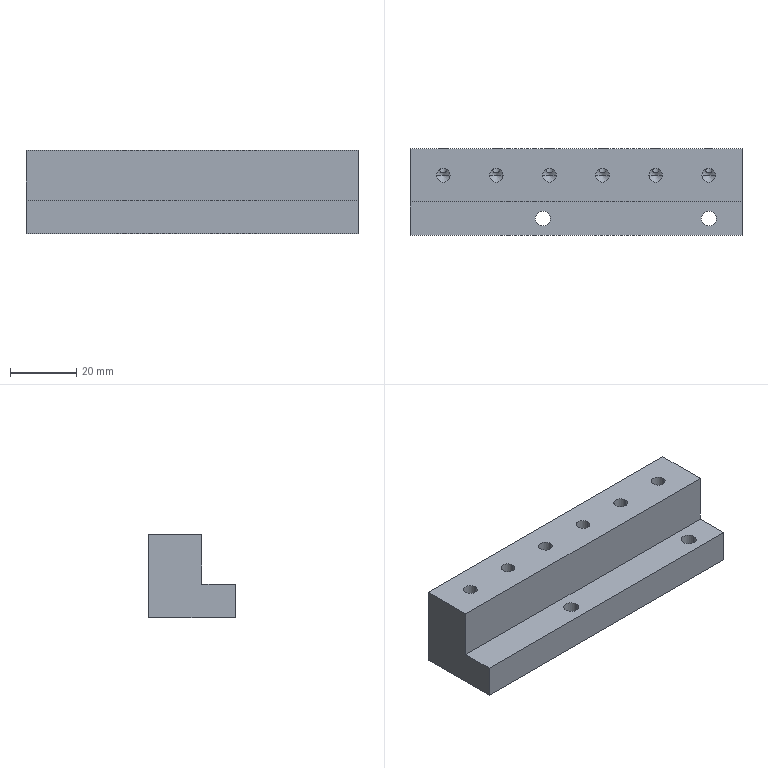Part | SolidWorks | features BaseBody 1 | 1 solid | 48 faces | box 100 x 26 x 25 mm | volume 48829 mm3 | cylinder 28 | cone 12 | plane 8 | commonest cylinder face diameters 2.459 x12 4.134 x12 4.5 x4